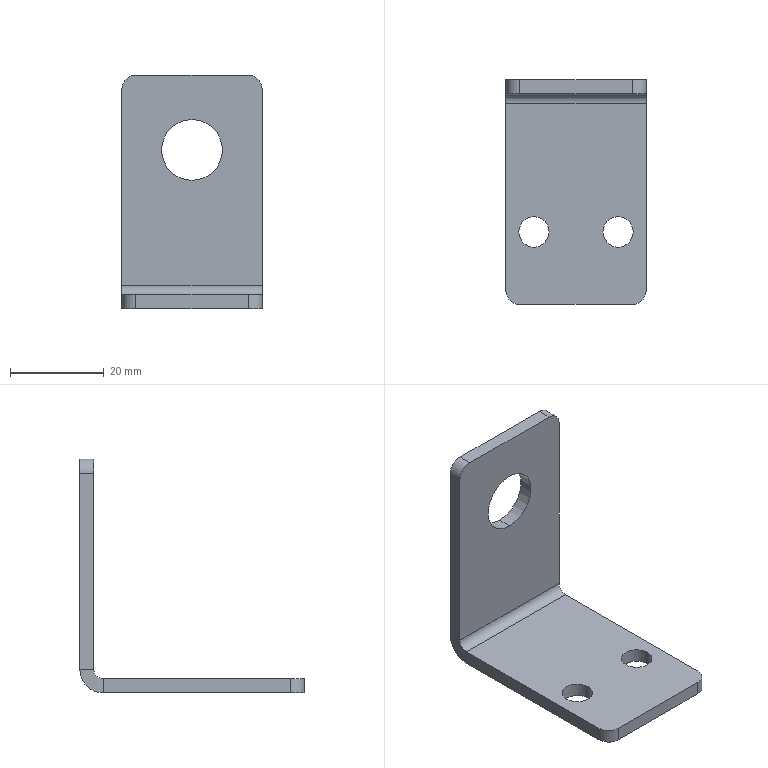Part | SolidWorks | features HoleWzd 2, Chamfer 1, EdgeFlange 1, Fillet 1, FlatPattern 1, ICE 1, SMBaseFlange 1, SheetMetal 1 | 1 solid | 24 faces | box 30 x 48 x 50 mm | volume 7794 mm3 | cylinder 12 | plane 12 | commonest cylinder face diameters 6 x4 6.5 x4 13 x2 4 x1 10 x1
STEP:
#1=CARTESIAN_POINT('',(-12.25,-8.5,-3.));
#2=VERTEX_POINT('',#1);
#3=CARTESIAN_POINT('',(-5.75,-8.5,-3.));
#4=VERTEX_POINT('',#3);
#5=CARTESIAN_POINT('',(-9.,-8.5,-3.));
#6=DIRECTION('',(0.,0.,1.));
#7=DIRECTION('',(1.,0.,0.));
#8=AXIS2_PLACEMENT_3D('',#5,#6,#7);
#9=CIRCLE('',#8,3.25);
#10=EDGE_CURVE('',#2,#4,#9,.T.);
#11=ORIENTED_EDGE('',*,*,#10,.F.);
#12=CARTESIAN_POINT('',(-12.25,-8.5,0.));
#13=VERTEX_POINT('',#12);
#14=CARTESIAN_POINT('',(-12.25,-8.5,0.));
#15=DIRECTION('',(0.,0.,1.));
#16=VECTOR('',#15,1000.);
#17=LINE('',#14,#16);
#18=EDGE_CURVE('',#2,#13,#17,.T.);
#19=ORIENTED_EDGE('',*,*,#18,.T.);
#20=CARTESIAN_POINT('',(-5.75,-8.5,0.));
#21=VERTEX_POINT('',#20);
#22=CARTESIAN_POINT('',(-9.,-8.5,0.));
#23=DIRECTION('',(0.,0.,1.));
#24=DIRECTION('',(1.,0.,0.));
#25=AXIS2_PLACEMENT_3D('',#22,#23,#24);
#26=CIRCLE('',#25,3.25);
#27=EDGE_CURVE('',#13,#21,#26,.T.);
#28=ORIENTED_EDGE('',*,*,#27,.T.);
#29=CARTESIAN_POINT('',(-5.75,-8.5,0.));
#30=DIRECTION('',(0.,0.,1.));
#31=VECTOR('',#30,1000.);
#32=LINE('',#29,#31);
#33=EDGE_CURVE('',#4,#21,#32,.T.);
#34=ORIENTED_EDGE('',*,*,#33,.F.);
#35=EDGE_LOOP('',(#11,#19,#28,#34));
#36=FACE_OUTER_BOUND('',#35,.T.);
#37=CARTESIAN_POINT('',(-9.,-8.5,0.));
#38=DIRECTION('',(0.,0.,1.));
#39=DIRECTION('',(1.,0.,0.));
#40=AXIS2_PLACEMENT_3D('',#37,#38,#39);
#41=CYLINDRICAL_SURFACE('',#40,3.25);
#42=ADVANCED_FACE('',(#36),#41,.F.);
#43=CARTESIAN_POINT('',(5.75,-8.5,-3.));
#44=VERTEX_POINT('',#43);
#45=CARTESIAN_POINT('',(12.25,-8.5,-3.));
#46=VERTEX_POINT('',#45);
#47=CARTESIAN_POINT('',(9.,-8.5,-3.));
#48=DIRECTION('',(0.,0.,1.));
#49=DIRECTION('',(1.,0.,0.));
#50=AXIS2_PLACEMENT_3D('',#47,#48,#49);
#51=CIRCLE('',#50,3.25);
#52=EDGE_CURVE('',#44,#46,#51,.T.);
#53=ORIENTED_EDGE('',*,*,#52,.F.);
#54=CARTESIAN_POINT('',(5.75,-8.5,0.));
#55=VERTEX_POINT('',#54);
#56=CARTESIAN_POINT('',(5.75,-8.5,0.));
#57=DIRECTION('',(0.,0.,1.));
#58=VECTOR('',#57,1000.);
#59=LINE('',#56,#58);
#60=EDGE_CURVE('',#44,#55,#59,.T.);
#61=ORIENTED_EDGE('',*,*,#60,.T.);
#62=CARTESIAN_POINT('',(12.25,-8.5,0.));
#63=VERTEX_POINT('',#62);
#64=CARTESIAN_POINT('',(9.,-8.5,0.));
#65=DIRECTION('',(0.,0.,1.));
#66=DIRECTION('',(1.,0.,0.));
#67=AXIS2_PLACEMENT_3D('',#64,#65,#66);
#68=CIRCLE('',#67,3.25);
#69=EDGE_CURVE('',#55,#63,#68,.T.);
#70=ORIENTED_EDGE('',*,*,#69,.T.);
#71=CARTESIAN_POINT('',(12.25,-8.5,0.));
#72=DIRECTION('',(0.,0.,1.));
#73=VECTOR('',#72,1000.);
#74=LINE('',#71,#73);
#75=EDGE_CURVE('',#46,#63,#74,.T.);
#76=ORIENTED_EDGE('',*,*,#75,.F.);
#77=EDGE_LOOP('',(#53,#61,#70,#76));
#78=FACE_OUTER_BOUND('',#77,.T.);
#79=CARTESIAN_POINT('',(9.,-8.5,0.));
#80=DIRECTION('',(0.,0.,1.));
#81=DIRECTION('',(1.,0.,0.));
#82=AXIS2_PLACEMENT_3D('',#79,#80,#81);
#83=CYLINDRICAL_SURFACE('',#82,3.25);
#84=ADVANCED_FACE('',(#78),#83,.F.);
#85=CARTESIAN_POINT('',(0.,24.,37.5));
#86=VERTEX_POINT('',#85);
#87=CARTESIAN_POINT('',(0.,24.,24.5));
#88=VERTEX_POINT('',#87);
#89=CARTESIAN_POINT('',(0.,24.,31.));
#90=DIRECTION('',(0.,-1.,0.));
#91=DIRECTION('',(0.,0.,-1.));
#92=AXIS2_PLACEMENT_3D('',#89,#90,#91);
#93=CIRCLE('',#92,6.5);
#94=EDGE_CURVE('',#86,#88,#93,.T.);
#95=ORIENTED_EDGE('',*,*,#94,.F.);
#96=CARTESIAN_POINT('',(0.,21.,37.5));
#97=VERTEX_POINT('',#96);
#98=CARTESIAN_POINT('',(0.,31.,37.5));
#99=DIRECTION('',(0.,-1.,0.));
#100=VECTOR('',#99,1000.);
#101=LINE('',#98,#100);
#102=EDGE_CURVE('',#86,#97,#101,.T.);
#103=ORIENTED_EDGE('',*,*,#102,.T.);
#104=CARTESIAN_POINT('',(0.,21.,24.5));
#105=VERTEX_POINT('',#104);
#106=CARTESIAN_POINT('',(0.,21.,31.));
#107=DIRECTION('',(0.,-1.,0.));
#108=DIRECTION('',(0.,0.,-1.));
#109=AXIS2_PLACEMENT_3D('',#106,#107,#108);
#110=CIRCLE('',#109,6.5);
#111=EDGE_CURVE('',#97,#105,#110,.T.);
#112=ORIENTED_EDGE('',*,*,#111,.T.);
#113=CARTESIAN_POINT('',(0.,31.,24.5));
#114=DIRECTION('',(0.,-1.,0.));
#115=VECTOR('',#114,1000.);
#116=LINE('',#113,#115);
#117=EDGE_CURVE('',#88,#105,#116,.T.);
#118=ORIENTED_EDGE('',*,*,#117,.F.);
#119=EDGE_LOOP('',(#95,#103,#112,#118));
#120=FACE_OUTER_BOUND('',#119,.T.);
#121=CARTESIAN_POINT('',(0.,31.,31.));
#122=DIRECTION('',(0.,-1.,0.));
#123=DIRECTION('',(0.,0.,-1.));
#124=AXIS2_PLACEMENT_3D('',#121,#122,#123);
#125=CYLINDRICAL_SURFACE('',#124,6.5);
#126=ADVANCED_FACE('',(#120),#125,.F.);
#127=CARTESIAN_POINT('',(-15.,19.,-3.));
#128=VERTEX_POINT('',#127);
#129=CARTESIAN_POINT('',(-15.,-21.,-3.));
#130=VERTEX_POINT('',#129);
#131=CARTESIAN_POINT('',(-15.,24.,-3.));
#132=DIRECTION('',(0.,-1.,0.));
#133=VECTOR('',#132,1000.);
#134=LINE('',#131,#133);
#135=EDGE_CURVE('',#128,#130,#134,.T.);
#136=ORIENTED_EDGE('',*,*,#135,.T.);
#137=CARTESIAN_POINT('',(-15.,-21.,0.));
#138=VERTEX_POINT('',#137);
#139=CARTESIAN_POINT('',(-15.,-21.,-3.));
#140=DIRECTION('',(0.,0.,1.));
#141=VECTOR('',#140,1000.);
#142=LINE('',#139,#141);
#143=EDGE_CURVE('',#130,#138,#142,.T.);
#144=ORIENTED_EDGE('',*,*,#143,.T.);
#145=CARTESIAN_POINT('',(-15.,19.,0.));
#146=VERTEX_POINT('',#145);
#147=CARTESIAN_POINT('',(-15.,24.,0.));
#148=DIRECTION('',(0.,-1.,0.));
#149=VECTOR('',#148,1000.);
#150=LINE('',#147,#149);
#151=EDGE_CURVE('',#146,#138,#150,.T.);
#152=ORIENTED_EDGE('',*,*,#151,.F.);
#153=CARTESIAN_POINT('',(-15.,19.,0.));
#154=DIRECTION('',(0.,0.,-1.));
#155=VECTOR('',#154,1000.);
#156=LINE('',#153,#155);
#157=EDGE_CURVE('',#146,#128,#156,.T.);
#158=ORIENTED_EDGE('',*,*,#157,.T.);
#159=EDGE_LOOP('',(#136,#144,#152,#158));
#160=FACE_OUTER_BOUND('',#159,.T.);
#161=CARTESIAN_POINT('',(-15.,24.,-3.));
#162=DIRECTION('',(-1.,0.,0.));
#163=DIRECTION('',(0.,-1.,0.));
#164=AXIS2_PLACEMENT_3D('',#161,#162,#163);
#165=PLANE('',#164);
#166=ADVANCED_FACE('',(#160),#165,.T.);
#167=CARTESIAN_POINT('',(-9.,-8.5,-3.));
#168=DIRECTION('',(0.,0.,1.));
#169=DIRECTION('',(1.,0.,0.));
#170=AXIS2_PLACEMENT_3D('',#167,#168,#169);
#171=CIRCLE('',#170,3.25);
#172=EDGE_CURVE('',#4,#2,#171,.T.);
#173=ORIENTED_EDGE('',*,*,#172,.T.);
#174=ORIENTED_EDGE('',*,*,#10,.T.);
#175=EDGE_LOOP('',(#173,#174));
#176=FACE_BOUND('',#175,.T.);
#177=CARTESIAN_POINT('',(9.,-8.5,-3.));
#178=DIRECTION('',(0.,0.,1.));
#179=DIRECTION('',(1.,0.,0.));
#180=AXIS2_PLACEMENT_3D('',#177,#178,#179);
#181=CIRCLE('',#180,3.25);
#182=EDGE_CURVE('',#46,#44,#181,.T.);
#183=ORIENTED_EDGE('',*,*,#182,.T.);
#184=ORIENTED_EDGE('',*,*,#52,.T.);
#185=EDGE_LOOP('',(#183,#184));
#186=FACE_BOUND('',#185,.T.);
#187=CARTESIAN_POINT('',(15.,-21.,-3.));
#188=VERTEX_POINT('',#187);
#189=CARTESIAN_POINT('',(15.,19.,-3.));
#190=VERTEX_POINT('',#189);
#191=CARTESIAN_POINT('',(15.,24.,-3.));
#192=DIRECTION('',(0.,1.,0.));
#193=VECTOR('',#192,1000.);
#194=LINE('',#191,#193);
#195=EDGE_CURVE('',#188,#190,#194,.T.);
#196=ORIENTED_EDGE('',*,*,#195,.F.);
#197=CARTESIAN_POINT('',(12.,-24.,-3.));
#198=VERTEX_POINT('',#197);
#199=CARTESIAN_POINT('',(12.,-21.,-3.));
#200=DIRECTION('',(0.,0.,-1.));
#201=DIRECTION('',(1.,0.,0.));
#202=AXIS2_PLACEMENT_3D('',#199,#200,#201);
#203=CIRCLE('',#202,3.);
#204=EDGE_CURVE('',#188,#198,#203,.T.);
#205=ORIENTED_EDGE('',*,*,#204,.T.);
#206=CARTESIAN_POINT('',(-12.,-24.,-3.));
#207=VERTEX_POINT('',#206);
#208=CARTESIAN_POINT('',(-15.,-24.,-3.));
#209=DIRECTION('',(1.,0.,0.));
#210=VECTOR('',#209,1000.);
#211=LINE('',#208,#210);
#212=EDGE_CURVE('',#207,#198,#211,.T.);
#213=ORIENTED_EDGE('',*,*,#212,.F.);
#214=CARTESIAN_POINT('',(-12.,-21.,-3.));
#215=DIRECTION('',(0.,0.,-1.));
#216=DIRECTION('',(1.,0.,0.));
#217=AXIS2_PLACEMENT_3D('',#214,#215,#216);
#218=CIRCLE('',#217,3.);
#219=EDGE_CURVE('',#207,#130,#218,.T.);
#220=ORIENTED_EDGE('',*,*,#219,.T.);
#221=ORIENTED_EDGE('',*,*,#135,.F.);
#222=CARTESIAN_POINT('',(-15.,19.,-3.));
#223=DIRECTION('',(1.,0.,0.));
#224=VECTOR('',#223,1000.);
#225=LINE('',#222,#224);
#226=EDGE_CURVE('',#128,#190,#225,.T.);
#227=ORIENTED_EDGE('',*,*,#226,.T.);
#228=EDGE_LOOP('',(#196,#205,#213,#220,#221,#227));
#229=FACE_OUTER_BOUND('',#228,.T.);
#230=CARTESIAN_POINT('',(0.,0.,-3.));
#231=DIRECTION('',(0.,0.,1.));
#232=DIRECTION('',(1.,0.,0.));
#233=AXIS2_PLACEMENT_3D('',#230,#231,#232);
#234=PLANE('',#233);
#235=ADVANCED_FACE('',(#176,#186,#229),#234,.F.);
#236=CARTESIAN_POINT('',(-9.,-8.5,0.));
#237=DIRECTION('',(0.,0.,1.));
#238=DIRECTION('',(1.,0.,0.));
#239=AXIS2_PLACEMENT_3D('',#236,#237,#238);
#240=CIRCLE('',#239,3.25);
#241=EDGE_CURVE('',#21,#13,#240,.T.);
#242=ORIENTED_EDGE('',*,*,#241,.F.);
#243=ORIENTED_EDGE('',*,*,#27,.F.);
#244=EDGE_LOOP('',(#242,#243));
#245=FACE_BOUND('',#244,.T.);
#246=CARTESIAN_POINT('',(9.,-8.5,0.));
#247=DIRECTION('',(0.,0.,1.));
#248=DIRECTION('',(1.,0.,0.));
#249=AXIS2_PLACEMENT_3D('',#246,#247,#248);
#250=CIRCLE('',#249,3.25);
#251=EDGE_CURVE('',#63,#55,#250,.T.);
#252=ORIENTED_EDGE('',*,*,#251,.F.);
#253=ORIENTED_EDGE('',*,*,#69,.F.);
#254=EDGE_LOOP('',(#252,#253));
#255=FACE_BOUND('',#254,.T.);
#256=CARTESIAN_POINT('',(-12.,-24.,0.));
#257=VERTEX_POINT('',#256);
#258=CARTESIAN_POINT('',(12.,-24.,0.));
#259=VERTEX_POINT('',#258);
#260=CARTESIAN_POINT('',(-15.,-24.,0.));
#261=DIRECTION('',(1.,0.,0.));
#262=VECTOR('',#261,1000.);
#263=LINE('',#260,#262);
#264=EDGE_CURVE('',#257,#259,#263,.T.);
#265=ORIENTED_EDGE('',*,*,#264,.T.);
#266=CARTESIAN_POINT('',(15.,-21.,0.));
#267=VERTEX_POINT('',#266);
#268=CARTESIAN_POINT('',(12.,-21.,0.));
#269=DIRECTION('',(0.,0.,1.));
#270=DIRECTION('',(1.,0.,0.));
#271=AXIS2_PLACEMENT_3D('',#268,#269,#270);
#272=CIRCLE('',#271,3.);
#273=EDGE_CURVE('',#259,#267,#272,.T.);
#274=ORIENTED_EDGE('',*,*,#273,.T.);
#275=CARTESIAN_POINT('',(15.,19.,0.));
#276=VERTEX_POINT('',#275);
#277=CARTESIAN_POINT('',(15.,24.,0.));
#278=DIRECTION('',(0.,1.,0.));
#279=VECTOR('',#278,1000.);
#280=LINE('',#277,#279);
#281=EDGE_CURVE('',#267,#276,#280,.T.);
#282=ORIENTED_EDGE('',*,*,#281,.T.);
#283=CARTESIAN_POINT('',(-15.,19.,0.));
#284=DIRECTION('',(1.,0.,0.));
#285=VECTOR('',#284,1000.);
#286=LINE('',#283,#285);
#287=EDGE_CURVE('',#146,#276,#286,.T.);
#288=ORIENTED_EDGE('',*,*,#287,.F.);
#289=ORIENTED_EDGE('',*,*,#151,.T.);
#290=CARTESIAN_POINT('',(-12.,-21.,0.));
#291=DIRECTION('',(0.,0.,1.));
#292=DIRECTION('',(1.,0.,0.));
#293=AXIS2_PLACEMENT_3D('',#290,#291,#292);
#294=CIRCLE('',#293,3.);
#295=EDGE_CURVE('',#138,#257,#294,.T.);
#296=ORIENTED_EDGE('',*,*,#295,.T.);
#297=EDGE_LOOP('',(#265,#274,#282,#288,#289,#296));
#298=FACE_OUTER_BOUND('',#297,.T.);
#299=CARTESIAN_POINT('',(0.,0.,0.));
#300=DIRECTION('',(0.,0.,1.));
#301=DIRECTION('',(1.,0.,0.));
#302=AXIS2_PLACEMENT_3D('',#299,#300,#301);
#303=PLANE('',#302);
#304=ADVANCED_FACE('',(#245,#255,#298),#303,.T.);
#305=ORIENTED_EDGE('',*,*,#281,.F.);
#306=CARTESIAN_POINT('',(15.,-21.,-3.));
#307=DIRECTION('',(0.,0.,-1.));
#308=VECTOR('',#307,1000.);
#309=LINE('',#306,#308);
#310=EDGE_CURVE('',#267,#188,#309,.T.);
#311=ORIENTED_EDGE('',*,*,#310,.T.);
#312=ORIENTED_EDGE('',*,*,#195,.T.);
#313=CARTESIAN_POINT('',(15.,19.,0.));
#314=DIRECTION('',(0.,0.,-1.));
#315=VECTOR('',#314,1000.);
#316=LINE('',#313,#315);
#317=EDGE_CURVE('',#276,#190,#316,.T.);
#318=ORIENTED_EDGE('',*,*,#317,.F.);
#319=EDGE_LOOP('',(#305,#311,#312,#318));
#320=FACE_OUTER_BOUND('',#319,.T.);
#321=CARTESIAN_POINT('',(15.,24.,-3.));
#322=DIRECTION('',(1.,0.,0.));
#323=DIRECTION('',(0.,1.,0.));
#324=AXIS2_PLACEMENT_3D('',#321,#322,#323);
#325=PLANE('',#324);
#326=ADVANCED_FACE('',(#320),#325,.T.);
#327=ORIENTED_EDGE('',*,*,#212,.T.);
#328=CARTESIAN_POINT('',(12.,-24.,-3.));
#329=DIRECTION('',(0.,0.,1.));
#330=VECTOR('',#329,1000.);
#331=LINE('',#328,#330);
#332=EDGE_CURVE('',#198,#259,#331,.T.);
#333=ORIENTED_EDGE('',*,*,#332,.T.);
#334=ORIENTED_EDGE('',*,*,#264,.F.);
#335=CARTESIAN_POINT('',(-12.,-24.,-3.));
#336=DIRECTION('',(0.,0.,-1.));
#337=VECTOR('',#336,1000.);
#338=LINE('',#335,#337);
#339=EDGE_CURVE('',#257,#207,#338,.T.);
#340=ORIENTED_EDGE('',*,*,#339,.T.);
#341=EDGE_LOOP('',(#327,#333,#334,#340));
#342=FACE_OUTER_BOUND('',#341,.T.);
#343=CARTESIAN_POINT('',(-15.,-24.,-3.));
#344=DIRECTION('',(0.,-1.,0.));
#345=DIRECTION('',(0.,0.,-1.));
#346=AXIS2_PLACEMENT_3D('',#343,#344,#345);
#347=PLANE('',#346);
#348=ADVANCED_FACE('',(#342),#347,.T.);
#349=CARTESIAN_POINT('',(15.,21.,2.));
#350=VERTEX_POINT('',#349);
#351=CARTESIAN_POINT('',(15.,24.,2.));
#352=VERTEX_POINT('',#351);
#353=CARTESIAN_POINT('',(15.,24.,2.));
#354=DIRECTION('',(0.,1.,0.));
#355=VECTOR('',#354,1000.);
#356=LINE('',#353,#355);
#357=EDGE_CURVE('',#350,#352,#356,.T.);
#358=ORIENTED_EDGE('',*,*,#357,.F.);
#359=CARTESIAN_POINT('',(15.,19.,2.));
#360=DIRECTION('',(1.,0.,0.));
#361=DIRECTION('',(0.,0.,1.));
#362=AXIS2_PLACEMENT_3D('',#359,#360,#361);
#363=CIRCLE('',#362,2.);
#364=EDGE_CURVE('',#276,#350,#363,.T.);
#365=ORIENTED_EDGE('',*,*,#364,.F.);
#366=ORIENTED_EDGE('',*,*,#317,.T.);
#367=CARTESIAN_POINT('',(15.,19.,2.));
#368=DIRECTION('',(1.,0.,0.));
#369=DIRECTION('',(0.,0.,1.));
#370=AXIS2_PLACEMENT_3D('',#367,#368,#369);
#371=CIRCLE('',#370,5.);
#372=EDGE_CURVE('',#190,#352,#371,.T.);
#373=ORIENTED_EDGE('',*,*,#372,.T.);
#374=EDGE_LOOP('',(#358,#365,#366,#373));
#375=FACE_OUTER_BOUND('',#374,.T.);
#376=CARTESIAN_POINT('',(15.,19.,2.));
#377=DIRECTION('',(1.,0.,0.));
#378=DIRECTION('',(0.,0.,-1.));
#379=AXIS2_PLACEMENT_3D('',#376,#377,#378);
#380=PLANE('',#379);
#381=ADVANCED_FACE('',(#375),#380,.T.);
#382=CARTESIAN_POINT('',(-15.,21.,2.));
#383=VERTEX_POINT('',#382);
#384=CARTESIAN_POINT('',(-15.,19.,2.));
#385=DIRECTION('',(-1.,0.,0.));
#386=DIRECTION('',(0.,0.,1.));
#387=AXIS2_PLACEMENT_3D('',#384,#385,#386);
#388=CIRCLE('',#387,2.);
#389=EDGE_CURVE('',#383,#146,#388,.T.);
#390=ORIENTED_EDGE('',*,*,#389,.F.);
#391=CARTESIAN_POINT('',(-15.,24.,2.));
#392=VERTEX_POINT('',#391);
#393=CARTESIAN_POINT('',(-15.,21.,2.));
#394=DIRECTION('',(0.,1.,0.));
#395=VECTOR('',#394,1000.);
#396=LINE('',#393,#395);
#397=EDGE_CURVE('',#383,#392,#396,.T.);
#398=ORIENTED_EDGE('',*,*,#397,.T.);
#399=CARTESIAN_POINT('',(-15.,19.,2.));
#400=DIRECTION('',(-1.,0.,0.));
#401=DIRECTION('',(0.,0.,1.));
#402=AXIS2_PLACEMENT_3D('',#399,#400,#401);
#403=CIRCLE('',#402,5.);
#404=EDGE_CURVE('',#392,#128,#403,.T.);
#405=ORIENTED_EDGE('',*,*,#404,.T.);
#406=ORIENTED_EDGE('',*,*,#157,.F.);
#407=EDGE_LOOP('',(#390,#398,#405,#406));
#408=FACE_OUTER_BOUND('',#407,.T.);
#409=CARTESIAN_POINT('',(-15.,19.,2.));
#410=DIRECTION('',(1.,0.,0.));
#411=DIRECTION('',(0.,0.,-1.));
#412=AXIS2_PLACEMENT_3D('',#409,#410,#411);
#413=PLANE('',#412);
#414=ADVANCED_FACE('',(#408),#413,.F.);
#415=ORIENTED_EDGE('',*,*,#226,.F.);
#416=ORIENTED_EDGE('',*,*,#404,.F.);
#417=CARTESIAN_POINT('',(15.,24.,2.));
#418=DIRECTION('',(1.,0.,0.));
#419=VECTOR('',#418,1000.);
#420=LINE('',#417,#419);
#421=EDGE_CURVE('',#392,#352,#420,.T.);
#422=ORIENTED_EDGE('',*,*,#421,.T.);
#423=ORIENTED_EDGE('',*,*,#372,.F.);
#424=EDGE_LOOP('',(#415,#416,#422,#423));
#425=FACE_OUTER_BOUND('',#424,.T.);
#426=CARTESIAN_POINT('',(-15.,19.,2.));
#427=DIRECTION('',(-1.,0.,0.));
#428=DIRECTION('',(0.,1.,0.));
#429=AXIS2_PLACEMENT_3D('',#426,#427,#428);
#430=CYLINDRICAL_SURFACE('',#429,5.);
#431=ADVANCED_FACE('',(#425),#430,.T.);
#432=ORIENTED_EDGE('',*,*,#287,.T.);
#433=ORIENTED_EDGE('',*,*,#364,.T.);
#434=CARTESIAN_POINT('',(15.,21.,2.));
#435=DIRECTION('',(-1.,0.,0.));
#436=VECTOR('',#435,1000.);
#437=LINE('',#434,#436);
#438=EDGE_CURVE('',#350,#383,#437,.T.);
#439=ORIENTED_EDGE('',*,*,#438,.T.);
#440=ORIENTED_EDGE('',*,*,#389,.T.);
#441=EDGE_LOOP('',(#432,#433,#439,#440));
#442=FACE_OUTER_BOUND('',#441,.T.);
#443=CARTESIAN_POINT('',(-15.,19.,2.));
#444=DIRECTION('',(-1.,0.,0.));
#445=DIRECTION('',(0.,1.,0.));
#446=AXIS2_PLACEMENT_3D('',#443,#444,#445);
#447=CYLINDRICAL_SURFACE('',#446,2.);
#448=ADVANCED_FACE('',(#442),#447,.F.);
#449=CARTESIAN_POINT('',(15.,24.,44.));
#450=VERTEX_POINT('',#449);
#451=CARTESIAN_POINT('',(15.,24.,0.));
#452=DIRECTION('',(0.,0.,-1.));
#453=VECTOR('',#452,1000.);
#454=LINE('',#451,#453);
#455=EDGE_CURVE('',#450,#352,#454,.T.);
#456=ORIENTED_EDGE('',*,*,#455,.F.);
#457=CARTESIAN_POINT('',(15.,21.,44.));
#458=VERTEX_POINT('',#457);
#459=CARTESIAN_POINT('',(15.,24.,44.));
#460=DIRECTION('',(0.,-1.,0.));
#461=VECTOR('',#460,1000.);
#462=LINE('',#459,#461);
#463=EDGE_CURVE('',#450,#458,#462,.T.);
#464=ORIENTED_EDGE('',*,*,#463,.T.);
#465=CARTESIAN_POINT('',(15.,21.,0.));
#466=DIRECTION('',(0.,0.,-1.));
#467=VECTOR('',#466,1000.);
#468=LINE('',#465,#467);
#469=EDGE_CURVE('',#458,#350,#468,.T.);
#470=ORIENTED_EDGE('',*,*,#469,.T.);
#471=ORIENTED_EDGE('',*,*,#357,.T.);
#472=EDGE_LOOP('',(#456,#464,#470,#471));
#473=FACE_OUTER_BOUND('',#472,.T.);
#474=CARTESIAN_POINT('',(15.,24.,0.));
#475=DIRECTION('',(-1.,0.,0.));
#476=DIRECTION('',(0.,0.,1.));
#477=AXIS2_PLACEMENT_3D('',#474,#475,#476);
#478=PLANE('',#477);
#479=ADVANCED_FACE('',(#473),#478,.F.);
#480=CARTESIAN_POINT('',(-15.,21.,44.));
#481=VERTEX_POINT('',#480);
#482=CARTESIAN_POINT('',(-15.,21.,47.));
#483=DIRECTION('',(0.,0.,1.));
#484=VECTOR('',#483,1000.);
#485=LINE('',#482,#484);
#486=EDGE_CURVE('',#383,#481,#485,.T.);
#487=ORIENTED_EDGE('',*,*,#486,.T.);
#488=CARTESIAN_POINT('',(-15.,24.,44.));
#489=VERTEX_POINT('',#488);
#490=CARTESIAN_POINT('',(-15.,24.,44.));
#491=DIRECTION('',(0.,1.,0.));
#492=VECTOR('',#491,1000.);
#493=LINE('',#490,#492);
#494=EDGE_CURVE('',#481,#489,#493,.T.);
#495=ORIENTED_EDGE('',*,*,#494,.T.);
#496=CARTESIAN_POINT('',(-15.,24.,0.));
#497=DIRECTION('',(0.,0.,1.));
#498=VECTOR('',#497,1000.);
#499=LINE('',#496,#498);
#500=EDGE_CURVE('',#392,#489,#499,.T.);
#501=ORIENTED_EDGE('',*,*,#500,.F.);
#502=ORIENTED_EDGE('',*,*,#397,.F.);
#503=EDGE_LOOP('',(#487,#495,#501,#502));
#504=FACE_OUTER_BOUND('',#503,.T.);
#505=CARTESIAN_POINT('',(-15.,24.,47.));
#506=DIRECTION('',(1.,0.,0.));
#507=DIRECTION('',(0.,0.,-1.));
#508=AXIS2_PLACEMENT_3D('',#505,#506,#507);
#509=PLANE('',#508);
#510=ADVANCED_FACE('',(#504),#509,.F.);
#511=CARTESIAN_POINT('',(0.,24.,31.));
#512=DIRECTION('',(0.,-1.,0.));
#513=DIRECTION('',(0.,0.,-1.));
#514=AXIS2_PLACEMENT_3D('',#511,#512,#513);
#515=CIRCLE('',#514,6.5);
#516=EDGE_CURVE('',#88,#86,#515,.T.);
#517=ORIENTED_EDGE('',*,*,#516,.T.);
#518=ORIENTED_EDGE('',*,*,#94,.T.);
#519=EDGE_LOOP('',(#517,#518));
#520=FACE_BOUND('',#519,.T.);
#521=CARTESIAN_POINT('',(-12.,24.,47.));
#522=VERTEX_POINT('',#521);
#523=CARTESIAN_POINT('',(12.,24.,47.));
#524=VERTEX_POINT('',#523);
#525=CARTESIAN_POINT('',(0.,24.,47.));
#526=DIRECTION('',(1.,0.,0.));
#527=VECTOR('',#526,1000.);
#528=LINE('',#525,#527);
#529=EDGE_CURVE('',#522,#524,#528,.T.);
#530=ORIENTED_EDGE('',*,*,#529,.T.);
#531=CARTESIAN_POINT('',(12.,24.,44.));
#532=DIRECTION('',(0.,1.,0.));
#533=DIRECTION('',(0.,0.,-1.));
#534=AXIS2_PLACEMENT_3D('',#531,#532,#533);
#535=CIRCLE('',#534,3.);
#536=EDGE_CURVE('',#524,#450,#535,.T.);
#537=ORIENTED_EDGE('',*,*,#536,.T.);
#538=ORIENTED_EDGE('',*,*,#455,.T.);
#539=ORIENTED_EDGE('',*,*,#421,.F.);
#540=ORIENTED_EDGE('',*,*,#500,.T.);
#541=CARTESIAN_POINT('',(-12.,24.,44.));
#542=DIRECTION('',(0.,1.,0.));
#543=DIRECTION('',(0.,0.,-1.));
#544=AXIS2_PLACEMENT_3D('',#541,#542,#543);
#545=CIRCLE('',#544,3.);
#546=EDGE_CURVE('',#489,#522,#545,.T.);
#547=ORIENTED_EDGE('',*,*,#546,.T.);
#548=EDGE_LOOP('',(#530,#537,#538,#539,#540,#547));
#549=FACE_OUTER_BOUND('',#548,.T.);
#550=CARTESIAN_POINT('',(0.,24.,0.));
#551=DIRECTION('',(0.,-1.,0.));
#552=DIRECTION('',(0.,0.,-1.));
#553=AXIS2_PLACEMENT_3D('',#550,#551,#552);
#554=PLANE('',#553);
#555=ADVANCED_FACE('',(#520,#549),#554,.F.);
#556=CARTESIAN_POINT('',(0.,21.,31.));
#557=DIRECTION('',(0.,-1.,0.));
#558=DIRECTION('',(0.,0.,-1.));
#559=AXIS2_PLACEMENT_3D('',#556,#557,#558);
#560=CIRCLE('',#559,6.5);
#561=EDGE_CURVE('',#105,#97,#560,.T.);
#562=ORIENTED_EDGE('',*,*,#561,.F.);
#563=ORIENTED_EDGE('',*,*,#111,.F.);
#564=EDGE_LOOP('',(#562,#563));
#565=FACE_BOUND('',#564,.T.);
#566=ORIENTED_EDGE('',*,*,#469,.F.);
#567=CARTESIAN_POINT('',(12.,21.,47.));
#568=VERTEX_POINT('',#567);
#569=CARTESIAN_POINT('',(12.,21.,44.));
#570=DIRECTION('',(0.,-1.,0.));
#571=DIRECTION('',(0.,0.,-1.));
#572=AXIS2_PLACEMENT_3D('',#569,#570,#571);
#573=CIRCLE('',#572,3.);
#574=EDGE_CURVE('',#458,#568,#573,.T.);
#575=ORIENTED_EDGE('',*,*,#574,.T.);
#576=CARTESIAN_POINT('',(-12.,21.,47.));
#577=VERTEX_POINT('',#576);
#578=CARTESIAN_POINT('',(15.,21.,47.));
#579=DIRECTION('',(1.,0.,0.));
#580=VECTOR('',#579,1000.);
#581=LINE('',#578,#580);
#582=EDGE_CURVE('',#577,#568,#581,.T.);
#583=ORIENTED_EDGE('',*,*,#582,.F.);
#584=CARTESIAN_POINT('',(-12.,21.,44.));
#585=DIRECTION('',(0.,-1.,0.));
#586=DIRECTION('',(0.,0.,-1.));
#587=AXIS2_PLACEMENT_3D('',#584,#585,#586);
#588=CIRCLE('',#587,3.);
#589=EDGE_CURVE('',#577,#481,#588,.T.);
#590=ORIENTED_EDGE('',*,*,#589,.T.);
#591=ORIENTED_EDGE('',*,*,#486,.F.);
#592=ORIENTED_EDGE('',*,*,#438,.F.);
#593=EDGE_LOOP('',(#566,#575,#583,#590,#591,#592));
#594=FACE_OUTER_BOUND('',#593,.T.);
#595=CARTESIAN_POINT('',(0.,21.,0.));
#596=DIRECTION('',(0.,-1.,0.));
#597=DIRECTION('',(0.,0.,-1.));
#598=AXIS2_PLACEMENT_3D('',#595,#596,#597);
#599=PLANE('',#598);
#600=ADVANCED_FACE('',(#565,#594),#599,.T.);
#601=ORIENTED_EDGE('',*,*,#582,.T.);
#602=CARTESIAN_POINT('',(12.,24.,47.));
#603=DIRECTION('',(0.,1.,0.));
#604=VECTOR('',#603,1000.);
#605=LINE('',#602,#604);
#606=EDGE_CURVE('',#568,#524,#605,.T.);
#607=ORIENTED_EDGE('',*,*,#606,.T.);
#608=ORIENTED_EDGE('',*,*,#529,.F.);
#609=CARTESIAN_POINT('',(-12.,24.,47.));
#610=DIRECTION('',(0.,-1.,0.));
#611=VECTOR('',#610,1000.);
#612=LINE('',#609,#611);
#613=EDGE_CURVE('',#522,#577,#612,.T.);
#614=ORIENTED_EDGE('',*,*,#613,.T.);
#615=EDGE_LOOP('',(#601,#607,#608,#614));
#616=FACE_OUTER_BOUND('',#615,.T.);
#617=CARTESIAN_POINT('',(15.,24.,47.));
#618=DIRECTION('',(0.,0.,-1.));
#619=DIRECTION('',(0.,1.,0.));
#620=AXIS2_PLACEMENT_3D('',#617,#618,#619);
#621=PLANE('',#620);
#622=ADVANCED_FACE('',(#616),#621,.F.);
#623=ORIENTED_EDGE('',*,*,#102,.F.);
#624=ORIENTED_EDGE('',*,*,#516,.F.);
#625=ORIENTED_EDGE('',*,*,#117,.T.);
#626=ORIENTED_EDGE('',*,*,#561,.T.);
#627=EDGE_LOOP('',(#623,#624,#625,#626));
#628=FACE_OUTER_BOUND('',#627,.T.);
#629=CARTESIAN_POINT('',(0.,31.,31.));
#630=DIRECTION('',(0.,-1.,0.));
#631=DIRECTION('',(0.,0.,-1.));
#632=AXIS2_PLACEMENT_3D('',#629,#630,#631);
#633=CYLINDRICAL_SURFACE('',#632,6.5);
#634=ADVANCED_FACE('',(#628),#633,.F.);
#635=ORIENTED_EDGE('',*,*,#204,.F.);
#636=ORIENTED_EDGE('',*,*,#310,.F.);
#637=ORIENTED_EDGE('',*,*,#273,.F.);
#638=ORIENTED_EDGE('',*,*,#332,.F.);
#639=EDGE_LOOP('',(#635,#636,#637,#638));
#640=FACE_OUTER_BOUND('',#639,.T.);
#641=CARTESIAN_POINT('',(12.,-21.,-3.));
#642=DIRECTION('',(0.,0.,1.));
#643=DIRECTION('',(1.,0.,0.));
#644=AXIS2_PLACEMENT_3D('',#641,#642,#643);
#645=CYLINDRICAL_SURFACE('',#644,3.);
#646=ADVANCED_FACE('',(#640),#645,.T.);
#647=ORIENTED_EDGE('',*,*,#219,.F.);
#648=ORIENTED_EDGE('',*,*,#339,.F.);
#649=ORIENTED_EDGE('',*,*,#295,.F.);
#650=ORIENTED_EDGE('',*,*,#143,.F.);
#651=EDGE_LOOP('',(#647,#648,#649,#650));
#652=FACE_OUTER_BOUND('',#651,.T.);
#653=CARTESIAN_POINT('',(-12.,-21.,-3.));
#654=DIRECTION('',(0.,0.,1.));
#655=DIRECTION('',(1.,0.,0.));
#656=AXIS2_PLACEMENT_3D('',#653,#654,#655);
#657=CYLINDRICAL_SURFACE('',#656,3.);
#658=ADVANCED_FACE('',(#652),#657,.T.);
#659=ORIENTED_EDGE('',*,*,#536,.F.);
#660=ORIENTED_EDGE('',*,*,#606,.F.);
#661=ORIENTED_EDGE('',*,*,#574,.F.);
#662=ORIENTED_EDGE('',*,*,#463,.F.);
#663=EDGE_LOOP('',(#659,#660,#661,#662));
#664=FACE_OUTER_BOUND('',#663,.T.);
#665=CARTESIAN_POINT('',(12.,24.,44.));
#666=DIRECTION('',(0.,-1.,0.));
#667=DIRECTION('',(0.,0.,-1.));
#668=AXIS2_PLACEMENT_3D('',#665,#666,#667);
#669=CYLINDRICAL_SURFACE('',#668,3.);
#670=ADVANCED_FACE('',(#664),#669,.T.);
#671=ORIENTED_EDGE('',*,*,#546,.F.);
#672=ORIENTED_EDGE('',*,*,#494,.F.);
#673=ORIENTED_EDGE('',*,*,#589,.F.);
#674=ORIENTED_EDGE('',*,*,#613,.F.);
#675=EDGE_LOOP('',(#671,#672,#673,#674));
#676=FACE_OUTER_BOUND('',#675,.T.);
#677=CARTESIAN_POINT('',(-12.,24.,44.));
#678=DIRECTION('',(0.,-1.,0.));
#679=DIRECTION('',(0.,0.,-1.));
#680=AXIS2_PLACEMENT_3D('',#677,#678,#679);
#681=CYLINDRICAL_SURFACE('',#680,3.);
#682=ADVANCED_FACE('',(#676),#681,.T.);
#683=ORIENTED_EDGE('',*,*,#60,.F.);
#684=ORIENTED_EDGE('',*,*,#182,.F.);
#685=ORIENTED_EDGE('',*,*,#75,.T.);
#686=ORIENTED_EDGE('',*,*,#251,.T.);
#687=EDGE_LOOP('',(#683,#684,#685,#686));
#688=FACE_OUTER_BOUND('',#687,.T.);
#689=CARTESIAN_POINT('',(9.,-8.5,0.));
#690=DIRECTION('',(0.,0.,1.));
#691=DIRECTION('',(1.,0.,0.));
#692=AXIS2_PLACEMENT_3D('',#689,#690,#691);
#693=CYLINDRICAL_SURFACE('',#692,3.25);
#694=ADVANCED_FACE('',(#688),#693,.F.);
#695=ORIENTED_EDGE('',*,*,#18,.F.);
#696=ORIENTED_EDGE('',*,*,#172,.F.);
#697=ORIENTED_EDGE('',*,*,#33,.T.);
#698=ORIENTED_EDGE('',*,*,#241,.T.);
#699=EDGE_LOOP('',(#695,#696,#697,#698));
#700=FACE_OUTER_BOUND('',#699,.T.);
#701=CARTESIAN_POINT('',(-9.,-8.5,0.));
#702=DIRECTION('',(0.,0.,1.));
#703=DIRECTION('',(1.,0.,0.));
#704=AXIS2_PLACEMENT_3D('',#701,#702,#703);
#705=CYLINDRICAL_SURFACE('',#704,3.25);
#706=ADVANCED_FACE('',(#700),#705,.F.);
#707=CLOSED_SHELL('',(#42,#84,#126,#166,#235,#304,#326,#348,#381,#414,#431,#448,#479,#510,#555,#600,#622,#634,#646,#658,#670,#682,#694,#706));
#708=MANIFOLD_SOLID_BREP('',#707);
#709=CARTESIAN_POINT('',(0.,0.,0.));
#710=DIRECTION('',(0.,0.,1.));
#711=DIRECTION('',(1.,0.,0.));
#712=AXIS2_PLACEMENT_3D('',#709,#710,#711);
#713=(LENGTH_UNIT()NAMED_UNIT(*)SI_UNIT(.MILLI.,.METRE.));
#714=UNCERTAINTY_MEASURE_WITH_UNIT(LENGTH_MEASURE(0.00001),#713,'','');
#715=(NAMED_UNIT(*)PLANE_ANGLE_UNIT()SI_UNIT($,.RADIAN.));
#716=(NAMED_UNIT(*)SI_UNIT($,.STERADIAN.)SOLID_ANGLE_UNIT());
#717=(GEOMETRIC_REPRESENTATION_CONTEXT(3)GLOBAL_UNCERTAINTY_ASSIGNED_CONTEXT((#714))GLOBAL_UNIT_ASSIGNED_CONTEXT((#713,#715,#716))REPRESENTATION_CONTEXT('',''));
#718=ADVANCED_BREP_SHAPE_REPRESENTATION('',(#708,#712),#717);